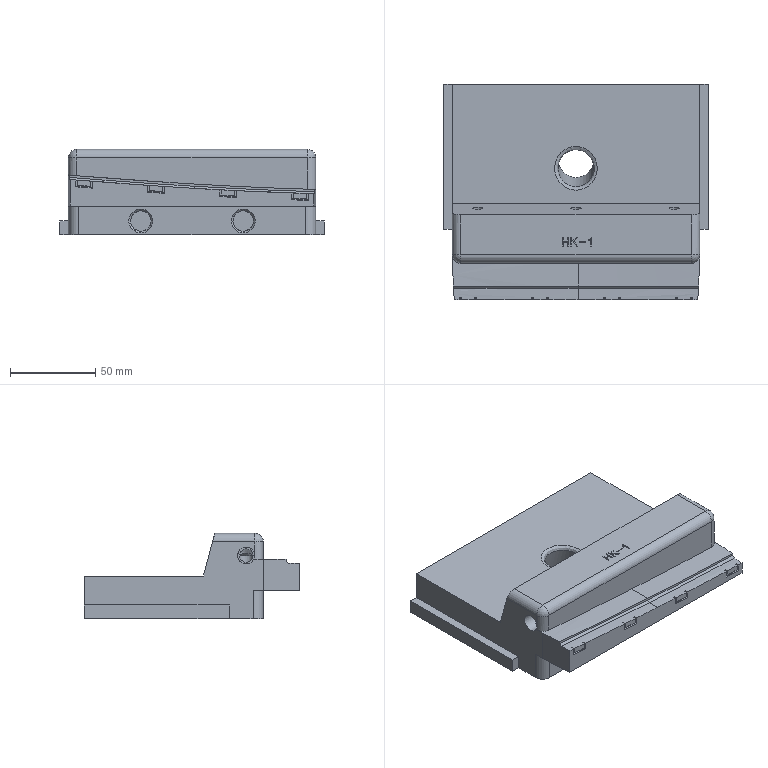Part | STEP file | solid 15 | 1 solid | 161 faces | box 155 x 126.362 x 50 mm | volume 501554 mm3 | plane 99 | cylinder 40 | cone 13 | torus 4 | sphere 2 | other 2 | spline 1 | commonest cylinder face diameters 10 x8 12 x8 8 x5 5 x3 6 x3 4377 x3